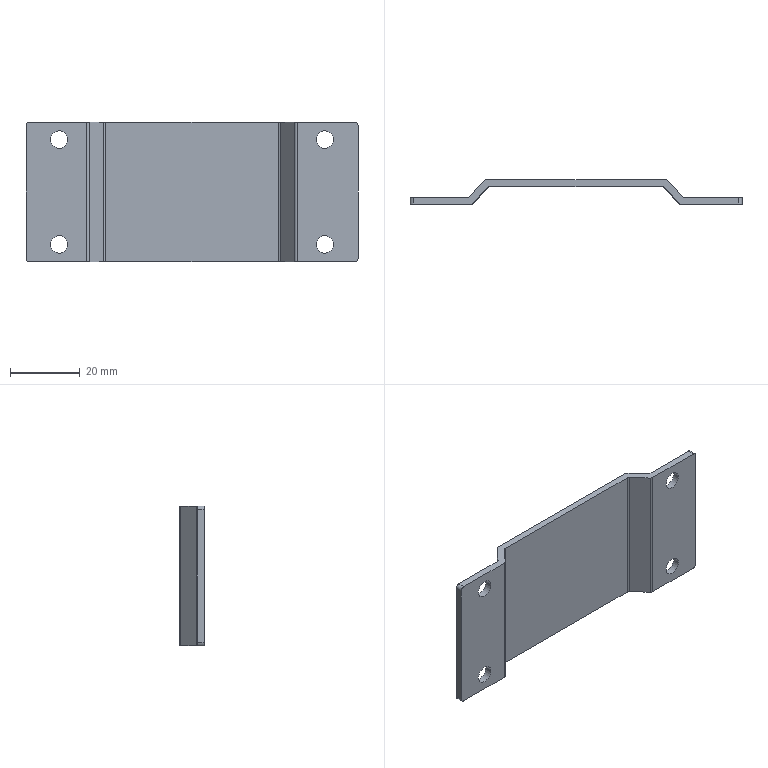Part | SolidWorks | features Extrusion 1, Fillet 1, ICE 1 | 1 solid | 34 faces | box 95 x 7 x 40 mm | volume 7797 mm3 | cylinder 20 | plane 14 | commonest cylinder face diameters 2 x12 5 x8
STEP:
#1=CARTESIAN_POINT('',(-40.5,-2.,15.));
#2=VERTEX_POINT('',#1);
#3=CARTESIAN_POINT('',(-35.5,-2.,15.));
#4=VERTEX_POINT('',#3);
#5=CARTESIAN_POINT('',(-38.,-2.,15.));
#6=DIRECTION('',(0.,-1.,0.));
#7=DIRECTION('',(0.,0.,-1.));
#8=AXIS2_PLACEMENT_3D('',#5,#6,#7);
#9=CIRCLE('',#8,2.5);
#10=EDGE_CURVE('',#2,#4,#9,.T.);
#11=ORIENTED_EDGE('',*,*,#10,.T.);
#12=CARTESIAN_POINT('',(-35.5,0.,15.));
#13=VERTEX_POINT('',#12);
#14=CARTESIAN_POINT('',(-35.5,-20.,15.));
#15=DIRECTION('',(0.,1.,0.));
#16=VECTOR('',#15,1000.);
#17=LINE('',#14,#16);
#18=EDGE_CURVE('',#4,#13,#17,.T.);
#19=ORIENTED_EDGE('',*,*,#18,.T.);
#20=CARTESIAN_POINT('',(-40.5,0.,15.));
#21=VERTEX_POINT('',#20);
#22=CARTESIAN_POINT('',(-38.,0.,15.));
#23=DIRECTION('',(0.,1.,0.));
#24=DIRECTION('',(1.,0.,0.));
#25=AXIS2_PLACEMENT_3D('',#22,#23,#24);
#26=CIRCLE('',#25,2.5);
#27=EDGE_CURVE('',#13,#21,#26,.T.);
#28=ORIENTED_EDGE('',*,*,#27,.T.);
#29=CARTESIAN_POINT('',(-40.5,-20.,15.));
#30=DIRECTION('',(0.,1.,0.));
#31=VECTOR('',#30,1000.);
#32=LINE('',#29,#31);
#33=EDGE_CURVE('',#2,#21,#32,.T.);
#34=ORIENTED_EDGE('',*,*,#33,.F.);
#35=EDGE_LOOP('',(#11,#19,#28,#34));
#36=FACE_OUTER_BOUND('',#35,.T.);
#37=CARTESIAN_POINT('',(-38.,-20.,15.));
#38=DIRECTION('',(0.,1.,0.));
#39=DIRECTION('',(-1.,0.,0.));
#40=AXIS2_PLACEMENT_3D('',#37,#38,#39);
#41=CYLINDRICAL_SURFACE('',#40,2.5);
#42=ADVANCED_FACE('',(#36),#41,.F.);
#43=CARTESIAN_POINT('',(35.5,-2.,15.));
#44=VERTEX_POINT('',#43);
#45=CARTESIAN_POINT('',(40.5,-2.,15.));
#46=VERTEX_POINT('',#45);
#47=CARTESIAN_POINT('',(38.,-2.,15.));
#48=DIRECTION('',(0.,-1.,0.));
#49=DIRECTION('',(0.,0.,-1.));
#50=AXIS2_PLACEMENT_3D('',#47,#48,#49);
#51=CIRCLE('',#50,2.5);
#52=EDGE_CURVE('',#44,#46,#51,.T.);
#53=ORIENTED_EDGE('',*,*,#52,.T.);
#54=CARTESIAN_POINT('',(40.5,0.,15.));
#55=VERTEX_POINT('',#54);
#56=CARTESIAN_POINT('',(40.5,-20.,15.));
#57=DIRECTION('',(0.,1.,0.));
#58=VECTOR('',#57,1000.);
#59=LINE('',#56,#58);
#60=EDGE_CURVE('',#46,#55,#59,.T.);
#61=ORIENTED_EDGE('',*,*,#60,.T.);
#62=CARTESIAN_POINT('',(35.5,0.,15.));
#63=VERTEX_POINT('',#62);
#64=CARTESIAN_POINT('',(38.,0.,15.));
#65=DIRECTION('',(0.,1.,0.));
#66=DIRECTION('',(-1.,0.,0.));
#67=AXIS2_PLACEMENT_3D('',#64,#65,#66);
#68=CIRCLE('',#67,2.5);
#69=EDGE_CURVE('',#55,#63,#68,.T.);
#70=ORIENTED_EDGE('',*,*,#69,.T.);
#71=CARTESIAN_POINT('',(35.5,-20.,15.));
#72=DIRECTION('',(0.,1.,0.));
#73=VECTOR('',#72,1000.);
#74=LINE('',#71,#73);
#75=EDGE_CURVE('',#44,#63,#74,.T.);
#76=ORIENTED_EDGE('',*,*,#75,.F.);
#77=EDGE_LOOP('',(#53,#61,#70,#76));
#78=FACE_OUTER_BOUND('',#77,.T.);
#79=CARTESIAN_POINT('',(38.,-20.,15.));
#80=DIRECTION('',(0.,1.,0.));
#81=DIRECTION('',(-1.,0.,0.));
#82=AXIS2_PLACEMENT_3D('',#79,#80,#81);
#83=CYLINDRICAL_SURFACE('',#82,2.5);
#84=ADVANCED_FACE('',(#78),#83,.F.);
#85=CARTESIAN_POINT('',(35.5,-2.,-15.));
#86=VERTEX_POINT('',#85);
#87=CARTESIAN_POINT('',(40.5,-2.,-15.));
#88=VERTEX_POINT('',#87);
#89=CARTESIAN_POINT('',(38.,-2.,-15.));
#90=DIRECTION('',(0.,-1.,0.));
#91=DIRECTION('',(0.,0.,-1.));
#92=AXIS2_PLACEMENT_3D('',#89,#90,#91);
#93=CIRCLE('',#92,2.5);
#94=EDGE_CURVE('',#86,#88,#93,.T.);
#95=ORIENTED_EDGE('',*,*,#94,.T.);
#96=CARTESIAN_POINT('',(40.5,0.,-15.));
#97=VERTEX_POINT('',#96);
#98=CARTESIAN_POINT('',(40.5,-20.,-15.));
#99=DIRECTION('',(0.,1.,0.));
#100=VECTOR('',#99,1000.);
#101=LINE('',#98,#100);
#102=EDGE_CURVE('',#88,#97,#101,.T.);
#103=ORIENTED_EDGE('',*,*,#102,.T.);
#104=CARTESIAN_POINT('',(35.5,0.,-15.));
#105=VERTEX_POINT('',#104);
#106=CARTESIAN_POINT('',(38.,0.,-15.));
#107=DIRECTION('',(0.,1.,0.));
#108=DIRECTION('',(1.,0.,0.));
#109=AXIS2_PLACEMENT_3D('',#106,#107,#108);
#110=CIRCLE('',#109,2.5);
#111=EDGE_CURVE('',#97,#105,#110,.T.);
#112=ORIENTED_EDGE('',*,*,#111,.T.);
#113=CARTESIAN_POINT('',(35.5,-20.,-15.));
#114=DIRECTION('',(0.,1.,0.));
#115=VECTOR('',#114,1000.);
#116=LINE('',#113,#115);
#117=EDGE_CURVE('',#86,#105,#116,.T.);
#118=ORIENTED_EDGE('',*,*,#117,.F.);
#119=EDGE_LOOP('',(#95,#103,#112,#118));
#120=FACE_OUTER_BOUND('',#119,.T.);
#121=CARTESIAN_POINT('',(38.,-20.,-15.));
#122=DIRECTION('',(0.,1.,0.));
#123=DIRECTION('',(-1.,0.,0.));
#124=AXIS2_PLACEMENT_3D('',#121,#122,#123);
#125=CYLINDRICAL_SURFACE('',#124,2.5);
#126=ADVANCED_FACE('',(#120),#125,.F.);
#127=CARTESIAN_POINT('',(-40.5,-2.,-15.));
#128=VERTEX_POINT('',#127);
#129=CARTESIAN_POINT('',(-35.5,-2.,-15.));
#130=VERTEX_POINT('',#129);
#131=CARTESIAN_POINT('',(-38.,-2.,-15.));
#132=DIRECTION('',(0.,-1.,0.));
#133=DIRECTION('',(0.,0.,-1.));
#134=AXIS2_PLACEMENT_3D('',#131,#132,#133);
#135=CIRCLE('',#134,2.5);
#136=EDGE_CURVE('',#128,#130,#135,.T.);
#137=ORIENTED_EDGE('',*,*,#136,.T.);
#138=CARTESIAN_POINT('',(-35.5,0.,-15.));
#139=VERTEX_POINT('',#138);
#140=CARTESIAN_POINT('',(-35.5,-20.,-15.));
#141=DIRECTION('',(0.,1.,0.));
#142=VECTOR('',#141,1000.);
#143=LINE('',#140,#142);
#144=EDGE_CURVE('',#130,#139,#143,.T.);
#145=ORIENTED_EDGE('',*,*,#144,.T.);
#146=CARTESIAN_POINT('',(-40.5,0.,-15.));
#147=VERTEX_POINT('',#146);
#148=CARTESIAN_POINT('',(-38.,0.,-15.));
#149=DIRECTION('',(0.,1.,0.));
#150=DIRECTION('',(-1.,0.,0.));
#151=AXIS2_PLACEMENT_3D('',#148,#149,#150);
#152=CIRCLE('',#151,2.5);
#153=EDGE_CURVE('',#139,#147,#152,.T.);
#154=ORIENTED_EDGE('',*,*,#153,.T.);
#155=CARTESIAN_POINT('',(-40.5,-20.,-15.));
#156=DIRECTION('',(0.,1.,0.));
#157=VECTOR('',#156,1000.);
#158=LINE('',#155,#157);
#159=EDGE_CURVE('',#128,#147,#158,.T.);
#160=ORIENTED_EDGE('',*,*,#159,.F.);
#161=EDGE_LOOP('',(#137,#145,#154,#160));
#162=FACE_OUTER_BOUND('',#161,.T.);
#163=CARTESIAN_POINT('',(-38.,-20.,-15.));
#164=DIRECTION('',(0.,1.,0.));
#165=DIRECTION('',(-1.,0.,0.));
#166=AXIS2_PLACEMENT_3D('',#163,#164,#165);
#167=CYLINDRICAL_SURFACE('',#166,2.5);
#168=ADVANCED_FACE('',(#162),#167,.F.);
#169=CARTESIAN_POINT('',(-47.5,0.,-19.));
#170=VERTEX_POINT('',#169);
#171=CARTESIAN_POINT('',(-47.5,0.,19.));
#172=VERTEX_POINT('',#171);
#173=CARTESIAN_POINT('',(-47.5,0.,-20.));
#174=DIRECTION('',(0.,0.,1.));
#175=VECTOR('',#174,1000.);
#176=LINE('',#173,#175);
#177=EDGE_CURVE('',#170,#172,#176,.T.);
#178=ORIENTED_EDGE('',*,*,#177,.F.);
#179=CARTESIAN_POINT('',(-47.5,-2.,-19.));
#180=VERTEX_POINT('',#179);
#181=CARTESIAN_POINT('',(-47.5,-2.,-19.));
#182=DIRECTION('',(0.,-1.,0.));
#183=VECTOR('',#182,1000.);
#184=LINE('',#181,#183);
#185=EDGE_CURVE('',#170,#180,#184,.T.);
#186=ORIENTED_EDGE('',*,*,#185,.T.);
#187=CARTESIAN_POINT('',(-47.5,-2.,19.));
#188=VERTEX_POINT('',#187);
#189=CARTESIAN_POINT('',(-47.5,-2.,-20.));
#190=DIRECTION('',(0.,0.,1.));
#191=VECTOR('',#190,1000.);
#192=LINE('',#189,#191);
#193=EDGE_CURVE('',#180,#188,#192,.T.);
#194=ORIENTED_EDGE('',*,*,#193,.T.);
#195=CARTESIAN_POINT('',(-47.5,-2.,19.));
#196=DIRECTION('',(0.,1.,0.));
#197=VECTOR('',#196,1000.);
#198=LINE('',#195,#197);
#199=EDGE_CURVE('',#188,#172,#198,.T.);
#200=ORIENTED_EDGE('',*,*,#199,.T.);
#201=EDGE_LOOP('',(#178,#186,#194,#200));
#202=FACE_OUTER_BOUND('',#201,.T.);
#203=CARTESIAN_POINT('',(-47.5,-2.,-20.));
#204=DIRECTION('',(-1.,0.,0.));
#205=DIRECTION('',(0.,0.,1.));
#206=AXIS2_PLACEMENT_3D('',#203,#204,#205);
#207=PLANE('',#206);
#208=ADVANCED_FACE('',(#202),#207,.T.);
#209=CARTESIAN_POINT('',(-38.,0.,15.));
#210=DIRECTION('',(0.,1.,0.));
#211=DIRECTION('',(1.,0.,0.));
#212=AXIS2_PLACEMENT_3D('',#209,#210,#211);
#213=CIRCLE('',#212,2.5);
#214=EDGE_CURVE('',#21,#13,#213,.T.);
#215=ORIENTED_EDGE('',*,*,#214,.F.);
#216=ORIENTED_EDGE('',*,*,#27,.F.);
#217=EDGE_LOOP('',(#215,#216));
#218=FACE_BOUND('',#217,.T.);
#219=CARTESIAN_POINT('',(-38.,0.,-15.));
#220=DIRECTION('',(0.,1.,0.));
#221=DIRECTION('',(-1.,0.,0.));
#222=AXIS2_PLACEMENT_3D('',#219,#220,#221);
#223=CIRCLE('',#222,2.5);
#224=EDGE_CURVE('',#147,#139,#223,.T.);
#225=ORIENTED_EDGE('',*,*,#224,.F.);
#226=ORIENTED_EDGE('',*,*,#153,.F.);
#227=EDGE_LOOP('',(#225,#226));
#228=FACE_BOUND('',#227,.T.);
#229=CARTESIAN_POINT('',(-30.945,0.,-20.));
#230=VERTEX_POINT('',#229);
#231=CARTESIAN_POINT('',(-46.5,0.,-20.));
#232=VERTEX_POINT('',#231);
#233=CARTESIAN_POINT('',(-47.5,0.,-20.));
#234=DIRECTION('',(-1.,0.,0.));
#235=VECTOR('',#234,1000.);
#236=LINE('',#233,#235);
#237=EDGE_CURVE('',#230,#232,#236,.T.);
#238=ORIENTED_EDGE('',*,*,#237,.T.);
#239=CARTESIAN_POINT('',(-46.5,0.,-19.));
#240=DIRECTION('',(0.,1.,0.));
#241=DIRECTION('',(0.,0.,1.));
#242=AXIS2_PLACEMENT_3D('',#239,#240,#241);
#243=CIRCLE('',#242,1.);
#244=EDGE_CURVE('',#232,#170,#243,.T.);
#245=ORIENTED_EDGE('',*,*,#244,.T.);
#246=ORIENTED_EDGE('',*,*,#177,.T.);
#247=CARTESIAN_POINT('',(-46.5,0.,20.));
#248=VERTEX_POINT('',#247);
#249=CARTESIAN_POINT('',(-46.5,0.,19.));
#250=DIRECTION('',(0.,1.,0.));
#251=DIRECTION('',(0.,0.,1.));
#252=AXIS2_PLACEMENT_3D('',#249,#250,#251);
#253=CIRCLE('',#252,1.);
#254=EDGE_CURVE('',#172,#248,#253,.T.);
#255=ORIENTED_EDGE('',*,*,#254,.T.);
#256=CARTESIAN_POINT('',(-30.945,0.,20.));
#257=VERTEX_POINT('',#256);
#258=CARTESIAN_POINT('',(-47.5,0.,20.));
#259=DIRECTION('',(-1.,0.,0.));
#260=VECTOR('',#259,1000.);
#261=LINE('',#258,#260);
#262=EDGE_CURVE('',#257,#248,#261,.T.);
#263=ORIENTED_EDGE('',*,*,#262,.F.);
#264=CARTESIAN_POINT('',(-30.945,0.,-20.));
#265=DIRECTION('',(0.,0.,1.));
#266=VECTOR('',#265,1000.);
#267=LINE('',#264,#266);
#268=EDGE_CURVE('',#230,#257,#267,.T.);
#269=ORIENTED_EDGE('',*,*,#268,.F.);
#270=EDGE_LOOP('',(#238,#245,#246,#255,#263,#269));
#271=FACE_OUTER_BOUND('',#270,.T.);
#272=CARTESIAN_POINT('',(-47.5,0.,-20.));
#273=DIRECTION('',(0.,1.,0.));
#274=DIRECTION('',(0.,0.,1.));
#275=AXIS2_PLACEMENT_3D('',#272,#273,#274);
#276=PLANE('',#275);
#277=ADVANCED_FACE('',(#218,#228,#271),#276,.T.);
#278=ORIENTED_EDGE('',*,*,#268,.T.);
#279=CARTESIAN_POINT('',(-30.202,0.331,20.));
#280=VERTEX_POINT('',#279);
#281=CARTESIAN_POINT('',(-30.945,1.,20.));
#282=DIRECTION('',(0.,0.,-1.));
#283=DIRECTION('',(1.,0.,0.));
#284=AXIS2_PLACEMENT_3D('',#281,#282,#283);
#285=CIRCLE('',#284,1.);
#286=EDGE_CURVE('',#280,#257,#285,.T.);
#287=ORIENTED_EDGE('',*,*,#286,.F.);
#288=CARTESIAN_POINT('',(-30.202,0.331,-20.));
#289=VERTEX_POINT('',#288);
#290=CARTESIAN_POINT('',(-30.202,0.331,-20.));
#291=DIRECTION('',(0.,0.,1.));
#292=VECTOR('',#291,1000.);
#293=LINE('',#290,#292);
#294=EDGE_CURVE('',#289,#280,#293,.T.);
#295=ORIENTED_EDGE('',*,*,#294,.F.);
#296=CARTESIAN_POINT('',(-30.945,1.,-20.));
#297=DIRECTION('',(0.,0.,-1.));
#298=DIRECTION('',(1.,0.,0.));
#299=AXIS2_PLACEMENT_3D('',#296,#297,#298);
#300=CIRCLE('',#299,1.);
#301=EDGE_CURVE('',#289,#230,#300,.T.);
#302=ORIENTED_EDGE('',*,*,#301,.T.);
#303=EDGE_LOOP('',(#278,#287,#295,#302));
#304=FACE_OUTER_BOUND('',#303,.T.);
#305=CARTESIAN_POINT('',(-30.945,1.,-20.));
#306=DIRECTION('',(0.,0.,1.));
#307=DIRECTION('',(1.,0.,0.));
#308=AXIS2_PLACEMENT_3D('',#305,#306,#307);
#309=CYLINDRICAL_SURFACE('',#308,1.);
#310=ADVANCED_FACE('',(#304),#309,.F.);
#311=ORIENTED_EDGE('',*,*,#294,.T.);
#312=CARTESIAN_POINT('',(-26.298,4.669,20.));
#313=VERTEX_POINT('',#312);
#314=CARTESIAN_POINT('',(-30.202,0.331,20.));
#315=DIRECTION('',(-0.669,-0.7433,0.));
#316=VECTOR('',#315,1000.);
#317=LINE('',#314,#316);
#318=EDGE_CURVE('',#313,#280,#317,.T.);
#319=ORIENTED_EDGE('',*,*,#318,.F.);
#320=CARTESIAN_POINT('',(-26.298,4.669,-20.));
#321=VERTEX_POINT('',#320);
#322=CARTESIAN_POINT('',(-26.298,4.669,-20.));
#323=DIRECTION('',(0.,0.,1.));
#324=VECTOR('',#323,1000.);
#325=LINE('',#322,#324);
#326=EDGE_CURVE('',#321,#313,#325,.T.);
#327=ORIENTED_EDGE('',*,*,#326,.F.);
#328=CARTESIAN_POINT('',(-30.202,0.331,-20.));
#329=DIRECTION('',(-0.669,-0.7433,0.));
#330=VECTOR('',#329,1000.);
#331=LINE('',#328,#330);
#332=EDGE_CURVE('',#321,#289,#331,.T.);
#333=ORIENTED_EDGE('',*,*,#332,.T.);
#334=EDGE_LOOP('',(#311,#319,#327,#333));
#335=FACE_OUTER_BOUND('',#334,.T.);
#336=CARTESIAN_POINT('',(-30.202,0.331,-20.));
#337=DIRECTION('',(-0.7433,0.669,0.));
#338=DIRECTION('',(-0.669,-0.7433,0.));
#339=AXIS2_PLACEMENT_3D('',#336,#337,#338);
#340=PLANE('',#339);
#341=ADVANCED_FACE('',(#335),#340,.T.);
#342=ORIENTED_EDGE('',*,*,#326,.T.);
#343=CARTESIAN_POINT('',(-25.555,5.,20.));
#344=VERTEX_POINT('',#343);
#345=CARTESIAN_POINT('',(-25.555,4.,20.));
#346=DIRECTION('',(0.,0.,1.));
#347=DIRECTION('',(-1.,0.,0.));
#348=AXIS2_PLACEMENT_3D('',#345,#346,#347);
#349=CIRCLE('',#348,1.);
#350=EDGE_CURVE('',#344,#313,#349,.T.);
#351=ORIENTED_EDGE('',*,*,#350,.F.);
#352=CARTESIAN_POINT('',(-25.555,5.,-20.));
#353=VERTEX_POINT('',#352);
#354=CARTESIAN_POINT('',(-25.555,5.,-20.));
#355=DIRECTION('',(0.,0.,1.));
#356=VECTOR('',#355,1000.);
#357=LINE('',#354,#356);
#358=EDGE_CURVE('',#353,#344,#357,.T.);
#359=ORIENTED_EDGE('',*,*,#358,.F.);
#360=CARTESIAN_POINT('',(-25.555,4.,-20.));
#361=DIRECTION('',(0.,0.,1.));
#362=DIRECTION('',(-1.,0.,0.));
#363=AXIS2_PLACEMENT_3D('',#360,#361,#362);
#364=CIRCLE('',#363,1.);
#365=EDGE_CURVE('',#353,#321,#364,.T.);
#366=ORIENTED_EDGE('',*,*,#365,.T.);
#367=EDGE_LOOP('',(#342,#351,#359,#366));
#368=FACE_OUTER_BOUND('',#367,.T.);
#369=CARTESIAN_POINT('',(-25.555,4.,-20.));
#370=DIRECTION('',(0.,0.,1.));
#371=DIRECTION('',(1.,0.,0.));
#372=AXIS2_PLACEMENT_3D('',#369,#370,#371);
#373=CYLINDRICAL_SURFACE('',#372,1.);
#374=ADVANCED_FACE('',(#368),#373,.T.);
#375=ORIENTED_EDGE('',*,*,#358,.T.);
#376=CARTESIAN_POINT('',(25.555,5.,20.));
#377=VERTEX_POINT('',#376);
#378=CARTESIAN_POINT('',(-25.555,5.,20.));
#379=DIRECTION('',(-1.,0.,0.));
#380=VECTOR('',#379,1000.);
#381=LINE('',#378,#380);
#382=EDGE_CURVE('',#377,#344,#381,.T.);
#383=ORIENTED_EDGE('',*,*,#382,.F.);
#384=CARTESIAN_POINT('',(25.555,5.,-20.));
#385=VERTEX_POINT('',#384);
#386=CARTESIAN_POINT('',(25.555,5.,-20.));
#387=DIRECTION('',(0.,0.,1.));
#388=VECTOR('',#387,1000.);
#389=LINE('',#386,#388);
#390=EDGE_CURVE('',#385,#377,#389,.T.);
#391=ORIENTED_EDGE('',*,*,#390,.F.);
#392=CARTESIAN_POINT('',(-25.555,5.,-20.));
#393=DIRECTION('',(-1.,0.,0.));
#394=VECTOR('',#393,1000.);
#395=LINE('',#392,#394);
#396=EDGE_CURVE('',#385,#353,#395,.T.);
#397=ORIENTED_EDGE('',*,*,#396,.T.);
#398=EDGE_LOOP('',(#375,#383,#391,#397));
#399=FACE_OUTER_BOUND('',#398,.T.);
#400=CARTESIAN_POINT('',(-25.555,5.,-20.));
#401=DIRECTION('',(0.,1.,0.));
#402=DIRECTION('',(0.,0.,1.));
#403=AXIS2_PLACEMENT_3D('',#400,#401,#402);
#404=PLANE('',#403);
#405=ADVANCED_FACE('',(#399),#404,.T.);
#406=ORIENTED_EDGE('',*,*,#390,.T.);
#407=CARTESIAN_POINT('',(26.298,4.669,20.));
#408=VERTEX_POINT('',#407);
#409=CARTESIAN_POINT('',(25.555,4.,20.));
#410=DIRECTION('',(0.,0.,1.));
#411=DIRECTION('',(-1.,0.,0.));
#412=AXIS2_PLACEMENT_3D('',#409,#410,#411);
#413=CIRCLE('',#412,1.);
#414=EDGE_CURVE('',#408,#377,#413,.T.);
#415=ORIENTED_EDGE('',*,*,#414,.F.);
#416=CARTESIAN_POINT('',(26.298,4.669,-20.));
#417=VERTEX_POINT('',#416);
#418=CARTESIAN_POINT('',(26.298,4.669,-20.));
#419=DIRECTION('',(0.,0.,1.));
#420=VECTOR('',#419,1000.);
#421=LINE('',#418,#420);
#422=EDGE_CURVE('',#417,#408,#421,.T.);
#423=ORIENTED_EDGE('',*,*,#422,.F.);
#424=CARTESIAN_POINT('',(25.555,4.,-20.));
#425=DIRECTION('',(0.,0.,1.));
#426=DIRECTION('',(-1.,0.,0.));
#427=AXIS2_PLACEMENT_3D('',#424,#425,#426);
#428=CIRCLE('',#427,1.);
#429=EDGE_CURVE('',#417,#385,#428,.T.);
#430=ORIENTED_EDGE('',*,*,#429,.T.);
#431=EDGE_LOOP('',(#406,#415,#423,#430));
#432=FACE_OUTER_BOUND('',#431,.T.);
#433=CARTESIAN_POINT('',(25.555,4.,-20.));
#434=DIRECTION('',(0.,0.,1.));
#435=DIRECTION('',(1.,0.,0.));
#436=AXIS2_PLACEMENT_3D('',#433,#434,#435);
#437=CYLINDRICAL_SURFACE('',#436,1.);
#438=ADVANCED_FACE('',(#432),#437,.T.);
#439=ORIENTED_EDGE('',*,*,#422,.T.);
#440=CARTESIAN_POINT('',(30.202,0.331,20.));
#441=VERTEX_POINT('',#440);
#442=CARTESIAN_POINT('',(26.298,4.669,20.));
#443=DIRECTION('',(-0.669,0.7433,0.));
#444=VECTOR('',#443,1000.);
#445=LINE('',#442,#444);
#446=EDGE_CURVE('',#441,#408,#445,.T.);
#447=ORIENTED_EDGE('',*,*,#446,.F.);
#448=CARTESIAN_POINT('',(30.202,0.331,-20.));
#449=VERTEX_POINT('',#448);
#450=CARTESIAN_POINT('',(30.202,0.331,-20.));
#451=DIRECTION('',(0.,0.,1.));
#452=VECTOR('',#451,1000.);
#453=LINE('',#450,#452);
#454=EDGE_CURVE('',#449,#441,#453,.T.);
#455=ORIENTED_EDGE('',*,*,#454,.F.);
#456=CARTESIAN_POINT('',(26.298,4.669,-20.));
#457=DIRECTION('',(-0.669,0.7433,0.));
#458=VECTOR('',#457,1000.);
#459=LINE('',#456,#458);
#460=EDGE_CURVE('',#449,#417,#459,.T.);
#461=ORIENTED_EDGE('',*,*,#460,.T.);
#462=EDGE_LOOP('',(#439,#447,#455,#461));
#463=FACE_OUTER_BOUND('',#462,.T.);
#464=CARTESIAN_POINT('',(26.298,4.669,-20.));
#465=DIRECTION('',(0.7433,0.669,0.));
#466=DIRECTION('',(-0.669,0.7433,0.));
#467=AXIS2_PLACEMENT_3D('',#464,#465,#466);
#468=PLANE('',#467);
#469=ADVANCED_FACE('',(#463),#468,.T.);
#470=ORIENTED_EDGE('',*,*,#454,.T.);
#471=CARTESIAN_POINT('',(30.945,0.,20.));
#472=VERTEX_POINT('',#471);
#473=CARTESIAN_POINT('',(30.945,1.,20.));
#474=DIRECTION('',(0.,0.,-1.));
#475=DIRECTION('',(1.,0.,0.));
#476=AXIS2_PLACEMENT_3D('',#473,#474,#475);
#477=CIRCLE('',#476,1.);
#478=EDGE_CURVE('',#472,#441,#477,.T.);
#479=ORIENTED_EDGE('',*,*,#478,.F.);
#480=CARTESIAN_POINT('',(30.945,0.,-20.));
#481=VERTEX_POINT('',#480);
#482=CARTESIAN_POINT('',(30.945,0.,-20.));
#483=DIRECTION('',(0.,0.,1.));
#484=VECTOR('',#483,1000.);
#485=LINE('',#482,#484);
#486=EDGE_CURVE('',#481,#472,#485,.T.);
#487=ORIENTED_EDGE('',*,*,#486,.F.);
#488=CARTESIAN_POINT('',(30.945,1.,-20.));
#489=DIRECTION('',(0.,0.,-1.));
#490=DIRECTION('',(1.,0.,0.));
#491=AXIS2_PLACEMENT_3D('',#488,#489,#490);
#492=CIRCLE('',#491,1.);
#493=EDGE_CURVE('',#481,#449,#492,.T.);
#494=ORIENTED_EDGE('',*,*,#493,.T.);
#495=EDGE_LOOP('',(#470,#479,#487,#494));
#496=FACE_OUTER_BOUND('',#495,.T.);
#497=CARTESIAN_POINT('',(30.945,1.,-20.));
#498=DIRECTION('',(0.,0.,1.));
#499=DIRECTION('',(1.,0.,0.));
#500=AXIS2_PLACEMENT_3D('',#497,#498,#499);
#501=CYLINDRICAL_SURFACE('',#500,1.);
#502=ADVANCED_FACE('',(#496),#501,.F.);
#503=CARTESIAN_POINT('',(38.,0.,15.));
#504=DIRECTION('',(0.,1.,0.));
#505=DIRECTION('',(-1.,0.,0.));
#506=AXIS2_PLACEMENT_3D('',#503,#504,#505);
#507=CIRCLE('',#506,2.5);
#508=EDGE_CURVE('',#63,#55,#507,.T.);
#509=ORIENTED_EDGE('',*,*,#508,.F.);
#510=ORIENTED_EDGE('',*,*,#69,.F.);
#511=EDGE_LOOP('',(#509,#510));
#512=FACE_BOUND('',#511,.T.);
#513=CARTESIAN_POINT('',(38.,0.,-15.));
#514=DIRECTION('',(0.,1.,0.));
#515=DIRECTION('',(1.,0.,0.));
#516=AXIS2_PLACEMENT_3D('',#513,#514,#515);
#517=CIRCLE('',#516,2.5);
#518=EDGE_CURVE('',#105,#97,#517,.T.);
#519=ORIENTED_EDGE('',*,*,#518,.F.);
#520=ORIENTED_EDGE('',*,*,#111,.F.);
#521=EDGE_LOOP('',(#519,#520));
#522=FACE_BOUND('',#521,.T.);
#523=CARTESIAN_POINT('',(47.5,0.,-19.));
#524=VERTEX_POINT('',#523);
#525=CARTESIAN_POINT('',(47.5,0.,19.));
#526=VERTEX_POINT('',#525);
#527=CARTESIAN_POINT('',(47.5,0.,-20.));
#528=DIRECTION('',(0.,0.,1.));
#529=VECTOR('',#528,1000.);
#530=LINE('',#527,#529);
#531=EDGE_CURVE('',#524,#526,#530,.T.);
#532=ORIENTED_EDGE('',*,*,#531,.F.);
#533=CARTESIAN_POINT('',(46.5,0.,-20.));
#534=VERTEX_POINT('',#533);
#535=CARTESIAN_POINT('',(46.5,0.,-19.));
#536=DIRECTION('',(0.,1.,0.));
#537=DIRECTION('',(-1.,0.,0.));
#538=AXIS2_PLACEMENT_3D('',#535,#536,#537);
#539=CIRCLE('',#538,1.);
#540=EDGE_CURVE('',#524,#534,#539,.T.);
#541=ORIENTED_EDGE('',*,*,#540,.T.);
#542=CARTESIAN_POINT('',(30.945,0.,-20.));
#543=DIRECTION('',(-1.,0.,0.));
#544=VECTOR('',#543,1000.);
#545=LINE('',#542,#544);
#546=EDGE_CURVE('',#534,#481,#545,.T.);
#547=ORIENTED_EDGE('',*,*,#546,.T.);
#548=ORIENTED_EDGE('',*,*,#486,.T.);
#549=CARTESIAN_POINT('',(46.5,0.,20.));
#550=VERTEX_POINT('',#549);
#551=CARTESIAN_POINT('',(30.945,0.,20.));
#552=DIRECTION('',(-1.,0.,0.));
#553=VECTOR('',#552,1000.);
#554=LINE('',#551,#553);
#555=EDGE_CURVE('',#550,#472,#554,.T.);
#556=ORIENTED_EDGE('',*,*,#555,.F.);
#557=CARTESIAN_POINT('',(46.5,0.,19.));
#558=DIRECTION('',(0.,1.,0.));
#559=DIRECTION('',(-1.,0.,0.));
#560=AXIS2_PLACEMENT_3D('',#557,#558,#559);
#561=CIRCLE('',#560,1.);
#562=EDGE_CURVE('',#550,#526,#561,.T.);
#563=ORIENTED_EDGE('',*,*,#562,.T.);
#564=EDGE_LOOP('',(#532,#541,#547,#548,#556,#563));
#565=FACE_OUTER_BOUND('',#564,.T.);
#566=CARTESIAN_POINT('',(30.945,0.,-20.));
#567=DIRECTION('',(0.,1.,0.));
#568=DIRECTION('',(-1.,0.,0.));
#569=AXIS2_PLACEMENT_3D('',#566,#567,#568);
#570=PLANE('',#569);
#571=ADVANCED_FACE('',(#512,#522,#565),#570,.T.);
#572=CARTESIAN_POINT('',(47.5,-2.,-19.));
#573=VERTEX_POINT('',#572);
#574=CARTESIAN_POINT('',(47.5,-2.,19.));
#575=VERTEX_POINT('',#574);
#576=CARTESIAN_POINT('',(47.5,-2.,-20.));
#577=DIRECTION('',(0.,0.,1.));
#578=VECTOR('',#577,1000.);
#579=LINE('',#576,#578);
#580=EDGE_CURVE('',#573,#575,#579,.T.);
#581=ORIENTED_EDGE('',*,*,#580,.F.);
#582=CARTESIAN_POINT('',(47.5,0.,-19.));
#583=DIRECTION('',(0.,1.,0.));
#584=VECTOR('',#583,1000.);
#585=LINE('',#582,#584);
#586=EDGE_CURVE('',#573,#524,#585,.T.);
#587=ORIENTED_EDGE('',*,*,#586,.T.);
#588=ORIENTED_EDGE('',*,*,#531,.T.);
#589=CARTESIAN_POINT('',(47.5,-2.,19.));
#590=DIRECTION('',(0.,-1.,0.));
#591=VECTOR('',#590,1000.);
#592=LINE('',#589,#591);
#593=EDGE_CURVE('',#526,#575,#592,.T.);
#594=ORIENTED_EDGE('',*,*,#593,.T.);
#595=EDGE_LOOP('',(#581,#587,#588,#594));
#596=FACE_OUTER_BOUND('',#595,.T.);
#597=CARTESIAN_POINT('',(47.5,-2.,-20.));
#598=DIRECTION('',(1.,0.,0.));
#599=DIRECTION('',(0.,0.,-1.));
#600=AXIS2_PLACEMENT_3D('',#597,#598,#599);
#601=PLANE('',#600);
#602=ADVANCED_FACE('',(#596),#601,.T.);
#603=ORIENTED_EDGE('',*,*,#52,.F.);
#604=CARTESIAN_POINT('',(38.,-2.,15.));
#605=DIRECTION('',(0.,-1.,0.));
#606=DIRECTION('',(0.,0.,-1.));
#607=AXIS2_PLACEMENT_3D('',#604,#605,#606);
#608=CIRCLE('',#607,2.5);
#609=EDGE_CURVE('',#46,#44,#608,.T.);
#610=ORIENTED_EDGE('',*,*,#609,.F.);
#611=EDGE_LOOP('',(#603,#610));
#612=FACE_BOUND('',#611,.T.);
#613=ORIENTED_EDGE('',*,*,#94,.F.);
#614=CARTESIAN_POINT('',(38.,-2.,-15.));
#615=DIRECTION('',(0.,-1.,0.));
#616=DIRECTION('',(0.,0.,-1.));
#617=AXIS2_PLACEMENT_3D('',#614,#615,#616);
#618=CIRCLE('',#617,2.5);
#619=EDGE_CURVE('',#88,#86,#618,.T.);
#620=ORIENTED_EDGE('',*,*,#619,.F.);
#621=EDGE_LOOP('',(#613,#620));
#622=FACE_BOUND('',#621,.T.);
#623=CARTESIAN_POINT('',(30.055,-2.,-20.));
#624=VERTEX_POINT('',#623);
#625=CARTESIAN_POINT('',(46.5,-2.,-20.));
#626=VERTEX_POINT('',#625);
#627=CARTESIAN_POINT('',(30.055,-2.,-20.));
#628=DIRECTION('',(1.,0.,0.));
#629=VECTOR('',#628,1000.);
#630=LINE('',#627,#629);
#631=EDGE_CURVE('',#624,#626,#630,.T.);
#632=ORIENTED_EDGE('',*,*,#631,.T.);
#633=CARTESIAN_POINT('',(46.5,-2.,-19.));
#634=DIRECTION('',(0.,-1.,0.));
#635=DIRECTION('',(0.,0.,-1.));
#636=AXIS2_PLACEMENT_3D('',#633,#634,#635);
#637=CIRCLE('',#636,1.);
#638=EDGE_CURVE('',#626,#573,#637,.T.);
#639=ORIENTED_EDGE('',*,*,#638,.T.);
#640=ORIENTED_EDGE('',*,*,#580,.T.);
#641=CARTESIAN_POINT('',(46.5,-2.,20.));
#642=VERTEX_POINT('',#641);
#643=CARTESIAN_POINT('',(46.5,-2.,19.));
#644=DIRECTION('',(0.,-1.,0.));
#645=DIRECTION('',(0.,0.,-1.));
#646=AXIS2_PLACEMENT_3D('',#643,#644,#645);
#647=CIRCLE('',#646,1.);
#648=EDGE_CURVE('',#575,#642,#647,.T.);
#649=ORIENTED_EDGE('',*,*,#648,.T.);
#650=CARTESIAN_POINT('',(30.055,-2.,20.));
#651=VERTEX_POINT('',#650);
#652=CARTESIAN_POINT('',(30.055,-2.,20.));
#653=DIRECTION('',(1.,0.,0.));
#654=VECTOR('',#653,1000.);
#655=LINE('',#652,#654);
#656=EDGE_CURVE('',#651,#642,#655,.T.);
#657=ORIENTED_EDGE('',*,*,#656,.F.);
#658=CARTESIAN_POINT('',(30.055,-2.,-20.));
#659=DIRECTION('',(0.,0.,1.));
#660=VECTOR('',#659,1000.);
#661=LINE('',#658,#660);
#662=EDGE_CURVE('',#624,#651,#661,.T.);
#663=ORIENTED_EDGE('',*,*,#662,.F.);
#664=EDGE_LOOP('',(#632,#639,#640,#649,#657,#663));
#665=FACE_OUTER_BOUND('',#664,.T.);
#666=CARTESIAN_POINT('',(30.055,-2.,-20.));
#667=DIRECTION('',(0.,-1.,0.));
#668=DIRECTION('',(0.,0.,-1.));
#669=AXIS2_PLACEMENT_3D('',#666,#667,#668);
#670=PLANE('',#669);
#671=ADVANCED_FACE('',(#612,#622,#665),#670,.T.);
#672=ORIENTED_EDGE('',*,*,#662,.T.);
#673=CARTESIAN_POINT('',(29.311,-1.669,20.));
#674=VERTEX_POINT('',#673);
#675=CARTESIAN_POINT('',(30.055,-1.,20.));
#676=DIRECTION('',(0.,0.,1.));
#677=DIRECTION('',(1.,0.,0.));
#678=AXIS2_PLACEMENT_3D('',#675,#676,#677);
#679=CIRCLE('',#678,1.);
#680=EDGE_CURVE('',#674,#651,#679,.T.);
#681=ORIENTED_EDGE('',*,*,#680,.F.);
#682=CARTESIAN_POINT('',(29.311,-1.669,-20.));
#683=VERTEX_POINT('',#682);
#684=CARTESIAN_POINT('',(29.311,-1.669,-20.));
#685=DIRECTION('',(0.,0.,1.));
#686=VECTOR('',#685,1000.);
#687=LINE('',#684,#686);
#688=EDGE_CURVE('',#683,#674,#687,.T.);
#689=ORIENTED_EDGE('',*,*,#688,.F.);
#690=CARTESIAN_POINT('',(30.055,-1.,-20.));
#691=DIRECTION('',(0.,0.,1.));
#692=DIRECTION('',(1.,0.,0.));
#693=AXIS2_PLACEMENT_3D('',#690,#691,#692);
#694=CIRCLE('',#693,1.);
#695=EDGE_CURVE('',#683,#624,#694,.T.);
#696=ORIENTED_EDGE('',*,*,#695,.T.);
#697=EDGE_LOOP('',(#672,#681,#689,#696));
#698=FACE_OUTER_BOUND('',#697,.T.);
#699=CARTESIAN_POINT('',(30.055,-1.,-20.));
#700=DIRECTION('',(0.,0.,1.));
#701=DIRECTION('',(1.,0.,0.));
#702=AXIS2_PLACEMENT_3D('',#699,#700,#701);
#703=CYLINDRICAL_SURFACE('',#702,1.);
#704=ADVANCED_FACE('',(#698),#703,.T.);
#705=ORIENTED_EDGE('',*,*,#688,.T.);
#706=CARTESIAN_POINT('',(25.407,2.669,20.));
#707=VERTEX_POINT('',#706);
#708=CARTESIAN_POINT('',(25.407,2.669,20.));
#709=DIRECTION('',(0.669,-0.7433,0.));
#710=VECTOR('',#709,1000.);
#711=LINE('',#708,#710);
#712=EDGE_CURVE('',#707,#674,#711,.T.);
#713=ORIENTED_EDGE('',*,*,#712,.F.);
#714=CARTESIAN_POINT('',(25.407,2.669,-20.));
#715=VERTEX_POINT('',#714);
#716=CARTESIAN_POINT('',(25.407,2.669,-20.));
#717=DIRECTION('',(0.,0.,1.));
#718=VECTOR('',#717,1000.);
#719=LINE('',#716,#718);
#720=EDGE_CURVE('',#715,#707,#719,.T.);
#721=ORIENTED_EDGE('',*,*,#720,.F.);
#722=CARTESIAN_POINT('',(25.407,2.669,-20.));
#723=DIRECTION('',(0.669,-0.7433,0.));
#724=VECTOR('',#723,1000.);
#725=LINE('',#722,#724);
#726=EDGE_CURVE('',#715,#683,#725,.T.);
#727=ORIENTED_EDGE('',*,*,#726,.T.);
#728=EDGE_LOOP('',(#705,#713,#721,#727));
#729=FACE_OUTER_BOUND('',#728,.T.);
#730=CARTESIAN_POINT('',(25.407,2.669,-20.));
#731=DIRECTION('',(-0.7433,-0.669,0.));
#732=DIRECTION('',(0.669,-0.7433,0.));
#733=AXIS2_PLACEMENT_3D('',#730,#731,#732);
#734=PLANE('',#733);
#735=ADVANCED_FACE('',(#729),#734,.T.);
#736=ORIENTED_EDGE('',*,*,#720,.T.);
#737=CARTESIAN_POINT('',(24.664,3.,20.));
#738=VERTEX_POINT('',#737);
#739=CARTESIAN_POINT('',(24.664,2.,20.));
#740=DIRECTION('',(0.,0.,-1.));
#741=DIRECTION('',(-1.,0.,0.));
#742=AXIS2_PLACEMENT_3D('',#739,#740,#741);
#743=CIRCLE('',#742,1.);
#744=EDGE_CURVE('',#738,#707,#743,.T.);
#745=ORIENTED_EDGE('',*,*,#744,.F.);
#746=CARTESIAN_POINT('',(24.664,3.,-20.));
#747=VERTEX_POINT('',#746);
#748=CARTESIAN_POINT('',(24.664,3.,-20.));
#749=DIRECTION('',(0.,0.,1.));
#750=VECTOR('',#749,1000.);
#751=LINE('',#748,#750);
#752=EDGE_CURVE('',#747,#738,#751,.T.);
#753=ORIENTED_EDGE('',*,*,#752,.F.);
#754=CARTESIAN_POINT('',(24.664,2.,-20.));
#755=DIRECTION('',(0.,0.,-1.));
#756=DIRECTION('',(-1.,0.,0.));
#757=AXIS2_PLACEMENT_3D('',#754,#755,#756);
#758=CIRCLE('',#757,1.);
#759=EDGE_CURVE('',#747,#715,#758,.T.);
#760=ORIENTED_EDGE('',*,*,#759,.T.);
#761=EDGE_LOOP('',(#736,#745,#753,#760));
#762=FACE_OUTER_BOUND('',#761,.T.);
#763=CARTESIAN_POINT('',(24.664,2.,-20.));
#764=DIRECTION('',(0.,0.,1.));
#765=DIRECTION('',(1.,0.,0.));
#766=AXIS2_PLACEMENT_3D('',#763,#764,#765);
#767=CYLINDRICAL_SURFACE('',#766,1.);
#768=ADVANCED_FACE('',(#762),#767,.F.);
#769=ORIENTED_EDGE('',*,*,#752,.T.);
#770=CARTESIAN_POINT('',(-24.664,3.,20.));
#771=VERTEX_POINT('',#770);
#772=CARTESIAN_POINT('',(-24.664,3.,20.));
#773=DIRECTION('',(1.,0.,0.));
#774=VECTOR('',#773,1000.);
#775=LINE('',#772,#774);
#776=EDGE_CURVE('',#771,#738,#775,.T.);
#777=ORIENTED_EDGE('',*,*,#776,.F.);
#778=CARTESIAN_POINT('',(-24.664,3.,-20.));
#779=VERTEX_POINT('',#778);
#780=CARTESIAN_POINT('',(-24.664,3.,-20.));
#781=DIRECTION('',(0.,0.,1.));
#782=VECTOR('',#781,1000.);
#783=LINE('',#780,#782);
#784=EDGE_CURVE('',#779,#771,#783,.T.);
#785=ORIENTED_EDGE('',*,*,#784,.F.);
#786=CARTESIAN_POINT('',(-24.664,3.,-20.));
#787=DIRECTION('',(1.,0.,0.));
#788=VECTOR('',#787,1000.);
#789=LINE('',#786,#788);
#790=EDGE_CURVE('',#779,#747,#789,.T.);
#791=ORIENTED_EDGE('',*,*,#790,.T.);
#792=EDGE_LOOP('',(#769,#777,#785,#791));
#793=FACE_OUTER_BOUND('',#792,.T.);
#794=CARTESIAN_POINT('',(-24.664,3.,-20.));
#795=DIRECTION('',(0.,-1.,0.));
#796=DIRECTION('',(0.,0.,-1.));
#797=AXIS2_PLACEMENT_3D('',#794,#795,#796);
#798=PLANE('',#797);
#799=ADVANCED_FACE('',(#793),#798,.T.);
#800=ORIENTED_EDGE('',*,*,#784,.T.);
#801=CARTESIAN_POINT('',(-25.407,2.669,20.));
#802=VERTEX_POINT('',#801);
#803=CARTESIAN_POINT('',(-24.664,2.,20.));
#804=DIRECTION('',(0.,0.,-1.));
#805=DIRECTION('',(-1.,0.,0.));
#806=AXIS2_PLACEMENT_3D('',#803,#804,#805);
#807=CIRCLE('',#806,1.);
#808=EDGE_CURVE('',#802,#771,#807,.T.);
#809=ORIENTED_EDGE('',*,*,#808,.F.);
#810=CARTESIAN_POINT('',(-25.407,2.669,-20.));
#811=VERTEX_POINT('',#810);
#812=CARTESIAN_POINT('',(-25.407,2.669,-20.));
#813=DIRECTION('',(0.,0.,1.));
#814=VECTOR('',#813,1000.);
#815=LINE('',#812,#814);
#816=EDGE_CURVE('',#811,#802,#815,.T.);
#817=ORIENTED_EDGE('',*,*,#816,.F.);
#818=CARTESIAN_POINT('',(-24.664,2.,-20.));
#819=DIRECTION('',(0.,0.,-1.));
#820=DIRECTION('',(-1.,0.,0.));
#821=AXIS2_PLACEMENT_3D('',#818,#819,#820);
#822=CIRCLE('',#821,1.);
#823=EDGE_CURVE('',#811,#779,#822,.T.);
#824=ORIENTED_EDGE('',*,*,#823,.T.);
#825=EDGE_LOOP('',(#800,#809,#817,#824));
#826=FACE_OUTER_BOUND('',#825,.T.);
#827=CARTESIAN_POINT('',(-24.664,2.,-20.));
#828=DIRECTION('',(0.,0.,1.));
#829=DIRECTION('',(1.,0.,0.));
#830=AXIS2_PLACEMENT_3D('',#827,#828,#829);
#831=CYLINDRICAL_SURFACE('',#830,1.);
#832=ADVANCED_FACE('',(#826),#831,.F.);
#833=ORIENTED_EDGE('',*,*,#816,.T.);
#834=CARTESIAN_POINT('',(-29.311,-1.669,20.));
#835=VERTEX_POINT('',#834);
#836=CARTESIAN_POINT('',(-29.311,-1.669,20.));
#837=DIRECTION('',(0.669,0.7433,0.));
#838=VECTOR('',#837,1000.);
#839=LINE('',#836,#838);
#840=EDGE_CURVE('',#835,#802,#839,.T.);
#841=ORIENTED_EDGE('',*,*,#840,.F.);
#842=CARTESIAN_POINT('',(-29.311,-1.669,-20.));
#843=VERTEX_POINT('',#842);
#844=CARTESIAN_POINT('',(-29.311,-1.669,-20.));
#845=DIRECTION('',(0.,0.,1.));
#846=VECTOR('',#845,1000.);
#847=LINE('',#844,#846);
#848=EDGE_CURVE('',#843,#835,#847,.T.);
#849=ORIENTED_EDGE('',*,*,#848,.F.);
#850=CARTESIAN_POINT('',(-29.311,-1.669,-20.));
#851=DIRECTION('',(0.669,0.7433,0.));
#852=VECTOR('',#851,1000.);
#853=LINE('',#850,#852);
#854=EDGE_CURVE('',#843,#811,#853,.T.);
#855=ORIENTED_EDGE('',*,*,#854,.T.);
#856=EDGE_LOOP('',(#833,#841,#849,#855));
#857=FACE_OUTER_BOUND('',#856,.T.);
#858=CARTESIAN_POINT('',(-29.311,-1.669,-20.));
#859=DIRECTION('',(0.7433,-0.669,0.));
#860=DIRECTION('',(0.669,0.7433,0.));
#861=AXIS2_PLACEMENT_3D('',#858,#859,#860);
#862=PLANE('',#861);
#863=ADVANCED_FACE('',(#857),#862,.T.);
#864=ORIENTED_EDGE('',*,*,#848,.T.);
#865=CARTESIAN_POINT('',(-30.055,-2.,20.));
#866=VERTEX_POINT('',#865);
#867=CARTESIAN_POINT('',(-30.055,-1.,20.));
#868=DIRECTION('',(0.,0.,1.));
#869=DIRECTION('',(1.,0.,0.));
#870=AXIS2_PLACEMENT_3D('',#867,#868,#869);
#871=CIRCLE('',#870,1.);
#872=EDGE_CURVE('',#866,#835,#871,.T.);
#873=ORIENTED_EDGE('',*,*,#872,.F.);
#874=CARTESIAN_POINT('',(-30.055,-2.,-20.));
#875=VERTEX_POINT('',#874);
#876=CARTESIAN_POINT('',(-30.055,-2.,-20.));
#877=DIRECTION('',(0.,0.,1.));
#878=VECTOR('',#877,1000.);
#879=LINE('',#876,#878);
#880=EDGE_CURVE('',#875,#866,#879,.T.);
#881=ORIENTED_EDGE('',*,*,#880,.F.);
#882=CARTESIAN_POINT('',(-30.055,-1.,-20.));
#883=DIRECTION('',(0.,0.,1.));
#884=DIRECTION('',(1.,0.,0.));
#885=AXIS2_PLACEMENT_3D('',#882,#883,#884);
#886=CIRCLE('',#885,1.);
#887=EDGE_CURVE('',#875,#843,#886,.T.);
#888=ORIENTED_EDGE('',*,*,#887,.T.);
#889=EDGE_LOOP('',(#864,#873,#881,#888));
#890=FACE_OUTER_BOUND('',#889,.T.);
#891=CARTESIAN_POINT('',(-30.055,-1.,-20.));
#892=DIRECTION('',(0.,0.,1.));
#893=DIRECTION('',(1.,0.,0.));
#894=AXIS2_PLACEMENT_3D('',#891,#892,#893);
#895=CYLINDRICAL_SURFACE('',#894,1.);
#896=ADVANCED_FACE('',(#890),#895,.T.);
#897=ORIENTED_EDGE('',*,*,#10,.F.);
#898=CARTESIAN_POINT('',(-38.,-2.,15.));
#899=DIRECTION('',(0.,-1.,0.));
#900=DIRECTION('',(0.,0.,-1.));
#901=AXIS2_PLACEMENT_3D('',#898,#899,#900);
#902=CIRCLE('',#901,2.5);
#903=EDGE_CURVE('',#4,#2,#902,.T.);
#904=ORIENTED_EDGE('',*,*,#903,.F.);
#905=EDGE_LOOP('',(#897,#904));
#906=FACE_BOUND('',#905,.T.);
#907=ORIENTED_EDGE('',*,*,#136,.F.);
#908=CARTESIAN_POINT('',(-38.,-2.,-15.));
#909=DIRECTION('',(0.,-1.,0.));
#910=DIRECTION('',(0.,0.,-1.));
#911=AXIS2_PLACEMENT_3D('',#908,#909,#910);
#912=CIRCLE('',#911,2.5);
#913=EDGE_CURVE('',#130,#128,#912,.T.);
#914=ORIENTED_EDGE('',*,*,#913,.F.);
#915=EDGE_LOOP('',(#907,#914));
#916=FACE_BOUND('',#915,.T.);
#917=ORIENTED_EDGE('',*,*,#193,.F.);
#918=CARTESIAN_POINT('',(-46.5,-2.,-20.));
#919=VERTEX_POINT('',#918);
#920=CARTESIAN_POINT('',(-46.5,-2.,-19.));
#921=DIRECTION('',(0.,-1.,0.));
#922=DIRECTION('',(0.,0.,-1.));
#923=AXIS2_PLACEMENT_3D('',#920,#921,#922);
#924=CIRCLE('',#923,1.);
#925=EDGE_CURVE('',#180,#919,#924,.T.);
#926=ORIENTED_EDGE('',*,*,#925,.T.);
#927=CARTESIAN_POINT('',(-47.5,-2.,-20.));
#928=DIRECTION('',(1.,0.,0.));
#929=VECTOR('',#928,1000.);
#930=LINE('',#927,#929);
#931=EDGE_CURVE('',#919,#875,#930,.T.);
#932=ORIENTED_EDGE('',*,*,#931,.T.);
#933=ORIENTED_EDGE('',*,*,#880,.T.);
#934=CARTESIAN_POINT('',(-46.5,-2.,20.));
#935=VERTEX_POINT('',#934);
#936=CARTESIAN_POINT('',(-47.5,-2.,20.));
#937=DIRECTION('',(1.,0.,0.));
#938=VECTOR('',#937,1000.);
#939=LINE('',#936,#938);
#940=EDGE_CURVE('',#935,#866,#939,.T.);
#941=ORIENTED_EDGE('',*,*,#940,.F.);
#942=CARTESIAN_POINT('',(-46.5,-2.,19.));
#943=DIRECTION('',(0.,-1.,0.));
#944=DIRECTION('',(0.,0.,-1.));
#945=AXIS2_PLACEMENT_3D('',#942,#943,#944);
#946=CIRCLE('',#945,1.);
#947=EDGE_CURVE('',#935,#188,#946,.T.);
#948=ORIENTED_EDGE('',*,*,#947,.T.);
#949=EDGE_LOOP('',(#917,#926,#932,#933,#941,#948));
#950=FACE_OUTER_BOUND('',#949,.T.);
#951=CARTESIAN_POINT('',(-47.5,-2.,-20.));
#952=DIRECTION('',(0.,-1.,0.));
#953=DIRECTION('',(0.,0.,-1.));
#954=AXIS2_PLACEMENT_3D('',#951,#952,#953);
#955=PLANE('',#954);
#956=ADVANCED_FACE('',(#906,#916,#950),#955,.T.);
#957=ORIENTED_EDGE('',*,*,#931,.F.);
#958=CARTESIAN_POINT('',(-46.5,0.,-20.));
#959=DIRECTION('',(0.,1.,0.));
#960=VECTOR('',#959,1000.);
#961=LINE('',#958,#960);
#962=EDGE_CURVE('',#919,#232,#961,.T.);
#963=ORIENTED_EDGE('',*,*,#962,.T.);
#964=ORIENTED_EDGE('',*,*,#237,.F.);
#965=ORIENTED_EDGE('',*,*,#301,.F.);
#966=ORIENTED_EDGE('',*,*,#332,.F.);
#967=ORIENTED_EDGE('',*,*,#365,.F.);
#968=ORIENTED_EDGE('',*,*,#396,.F.);
#969=ORIENTED_EDGE('',*,*,#429,.F.);
#970=ORIENTED_EDGE('',*,*,#460,.F.);
#971=ORIENTED_EDGE('',*,*,#493,.F.);
#972=ORIENTED_EDGE('',*,*,#546,.F.);
#973=CARTESIAN_POINT('',(46.5,-2.,-20.));
#974=DIRECTION('',(0.,-1.,0.));
#975=VECTOR('',#974,1000.);
#976=LINE('',#973,#975);
#977=EDGE_CURVE('',#534,#626,#976,.T.);
#978=ORIENTED_EDGE('',*,*,#977,.T.);
#979=ORIENTED_EDGE('',*,*,#631,.F.);
#980=ORIENTED_EDGE('',*,*,#695,.F.);
#981=ORIENTED_EDGE('',*,*,#726,.F.);
#982=ORIENTED_EDGE('',*,*,#759,.F.);
#983=ORIENTED_EDGE('',*,*,#790,.F.);
#984=ORIENTED_EDGE('',*,*,#823,.F.);
#985=ORIENTED_EDGE('',*,*,#854,.F.);
#986=ORIENTED_EDGE('',*,*,#887,.F.);
#987=EDGE_LOOP('',(#957,#963,#964,#965,#966,#967,#968,#969,#970,#971,#972,#978,#979,#980,#981,#982,#983,#984,#985,#986));
#988=FACE_OUTER_BOUND('',#987,.T.);
#989=CARTESIAN_POINT('',(-30.945,1.,-20.));
#990=DIRECTION('',(0.,0.,1.));
#991=DIRECTION('',(1.,0.,0.));
#992=AXIS2_PLACEMENT_3D('',#989,#990,#991);
#993=PLANE('',#992);
#994=ADVANCED_FACE('',(#988),#993,.F.);
#995=ORIENTED_EDGE('',*,*,#262,.T.);
#996=CARTESIAN_POINT('',(-46.5,1.,20.));
#997=DIRECTION('',(0.,-1.,0.));
#998=VECTOR('',#997,1000.);
#999=LINE('',#996,#998);
#1000=EDGE_CURVE('',#248,#935,#999,.T.);
#1001=ORIENTED_EDGE('',*,*,#1000,.T.);
#1002=ORIENTED_EDGE('',*,*,#940,.T.);
#1003=ORIENTED_EDGE('',*,*,#872,.T.);
#1004=ORIENTED_EDGE('',*,*,#840,.T.);
#1005=ORIENTED_EDGE('',*,*,#808,.T.);
#1006=ORIENTED_EDGE('',*,*,#776,.T.);
#1007=ORIENTED_EDGE('',*,*,#744,.T.);
#1008=ORIENTED_EDGE('',*,*,#712,.T.);
#1009=ORIENTED_EDGE('',*,*,#680,.T.);
#1010=ORIENTED_EDGE('',*,*,#656,.T.);
#1011=CARTESIAN_POINT('',(46.5,1.,20.));
#1012=DIRECTION('',(0.,1.,0.));
#1013=VECTOR('',#1012,1000.);
#1014=LINE('',#1011,#1013);
#1015=EDGE_CURVE('',#642,#550,#1014,.T.);
#1016=ORIENTED_EDGE('',*,*,#1015,.T.);
#1017=ORIENTED_EDGE('',*,*,#555,.T.);
#1018=ORIENTED_EDGE('',*,*,#478,.T.);
#1019=ORIENTED_EDGE('',*,*,#446,.T.);
#1020=ORIENTED_EDGE('',*,*,#414,.T.);
#1021=ORIENTED_EDGE('',*,*,#382,.T.);
#1022=ORIENTED_EDGE('',*,*,#350,.T.);
#1023=ORIENTED_EDGE('',*,*,#318,.T.);
#1024=ORIENTED_EDGE('',*,*,#286,.T.);
#1025=EDGE_LOOP('',(#995,#1001,#1002,#1003,#1004,#1005,#1006,#1007,#1008,#1009,#1010,#1016,#1017,#1018,#1019,#1020,#1021,#1022,#1023,#1024));
#1026=FACE_OUTER_BOUND('',#1025,.T.);
#1027=CARTESIAN_POINT('',(-30.945,1.,20.));
#1028=DIRECTION('',(0.,0.,1.));
#1029=DIRECTION('',(1.,0.,0.));
#1030=AXIS2_PLACEMENT_3D('',#1027,#1028,#1029);
#1031=PLANE('',#1030);
#1032=ADVANCED_FACE('',(#1026),#1031,.T.);
#1033=ORIENTED_EDGE('',*,*,#144,.F.);
#1034=ORIENTED_EDGE('',*,*,#913,.T.);
#1035=ORIENTED_EDGE('',*,*,#159,.T.);
#1036=ORIENTED_EDGE('',*,*,#224,.T.);
#1037=EDGE_LOOP('',(#1033,#1034,#1035,#1036));
#1038=FACE_OUTER_BOUND('',#1037,.T.);
#1039=CARTESIAN_POINT('',(-38.,-20.,-15.));
#1040=DIRECTION('',(0.,1.,0.));
#1041=DIRECTION('',(-1.,0.,0.));
#1042=AXIS2_PLACEMENT_3D('',#1039,#1040,#1041);
#1043=CYLINDRICAL_SURFACE('',#1042,2.5);
#1044=ADVANCED_FACE('',(#1038),#1043,.F.);
#1045=ORIENTED_EDGE('',*,*,#102,.F.);
#1046=ORIENTED_EDGE('',*,*,#619,.T.);
#1047=ORIENTED_EDGE('',*,*,#117,.T.);
#1048=ORIENTED_EDGE('',*,*,#518,.T.);
#1049=EDGE_LOOP('',(#1045,#1046,#1047,#1048));
#1050=FACE_OUTER_BOUND('',#1049,.T.);
#1051=CARTESIAN_POINT('',(38.,-20.,-15.));
#1052=DIRECTION('',(0.,1.,0.));
#1053=DIRECTION('',(-1.,0.,0.));
#1054=AXIS2_PLACEMENT_3D('',#1051,#1052,#1053);
#1055=CYLINDRICAL_SURFACE('',#1054,2.5);
#1056=ADVANCED_FACE('',(#1050),#1055,.F.);
#1057=ORIENTED_EDGE('',*,*,#60,.F.);
#1058=ORIENTED_EDGE('',*,*,#609,.T.);
#1059=ORIENTED_EDGE('',*,*,#75,.T.);
#1060=ORIENTED_EDGE('',*,*,#508,.T.);
#1061=EDGE_LOOP('',(#1057,#1058,#1059,#1060));
#1062=FACE_OUTER_BOUND('',#1061,.T.);
#1063=CARTESIAN_POINT('',(38.,-20.,15.));
#1064=DIRECTION('',(0.,1.,0.));
#1065=DIRECTION('',(-1.,0.,0.));
#1066=AXIS2_PLACEMENT_3D('',#1063,#1064,#1065);
#1067=CYLINDRICAL_SURFACE('',#1066,2.5);
#1068=ADVANCED_FACE('',(#1062),#1067,.F.);
#1069=ORIENTED_EDGE('',*,*,#18,.F.);
#1070=ORIENTED_EDGE('',*,*,#903,.T.);
#1071=ORIENTED_EDGE('',*,*,#33,.T.);
#1072=ORIENTED_EDGE('',*,*,#214,.T.);
#1073=EDGE_LOOP('',(#1069,#1070,#1071,#1072));
#1074=FACE_OUTER_BOUND('',#1073,.T.);
#1075=CARTESIAN_POINT('',(-38.,-20.,15.));
#1076=DIRECTION('',(0.,1.,0.));
#1077=DIRECTION('',(-1.,0.,0.));
#1078=AXIS2_PLACEMENT_3D('',#1075,#1076,#1077);
#1079=CYLINDRICAL_SURFACE('',#1078,2.5);
#1080=ADVANCED_FACE('',(#1074),#1079,.F.);
#1081=ORIENTED_EDGE('',*,*,#244,.F.);
#1082=ORIENTED_EDGE('',*,*,#962,.F.);
#1083=ORIENTED_EDGE('',*,*,#925,.F.);
#1084=ORIENTED_EDGE('',*,*,#185,.F.);
#1085=EDGE_LOOP('',(#1081,#1082,#1083,#1084));
#1086=FACE_OUTER_BOUND('',#1085,.T.);
#1087=CARTESIAN_POINT('',(-46.5,-2.,-19.));
#1088=DIRECTION('',(0.,1.,0.));
#1089=DIRECTION('',(0.,0.,1.));
#1090=AXIS2_PLACEMENT_3D('',#1087,#1088,#1089);
#1091=CYLINDRICAL_SURFACE('',#1090,1.);
#1092=ADVANCED_FACE('',(#1086),#1091,.T.);
#1093=ORIENTED_EDGE('',*,*,#254,.F.);
#1094=ORIENTED_EDGE('',*,*,#199,.F.);
#1095=ORIENTED_EDGE('',*,*,#947,.F.);
#1096=ORIENTED_EDGE('',*,*,#1000,.F.);
#1097=EDGE_LOOP('',(#1093,#1094,#1095,#1096));
#1098=FACE_OUTER_BOUND('',#1097,.T.);
#1099=CARTESIAN_POINT('',(-46.5,1.,19.));
#1100=DIRECTION('',(0.,-1.,0.));
#1101=DIRECTION('',(0.,0.,-1.));
#1102=AXIS2_PLACEMENT_3D('',#1099,#1100,#1101);
#1103=CYLINDRICAL_SURFACE('',#1102,1.);
#1104=ADVANCED_FACE('',(#1098),#1103,.T.);
#1105=ORIENTED_EDGE('',*,*,#638,.F.);
#1106=ORIENTED_EDGE('',*,*,#977,.F.);
#1107=ORIENTED_EDGE('',*,*,#540,.F.);
#1108=ORIENTED_EDGE('',*,*,#586,.F.);
#1109=EDGE_LOOP('',(#1105,#1106,#1107,#1108));
#1110=FACE_OUTER_BOUND('',#1109,.T.);
#1111=CARTESIAN_POINT('',(46.5,-2.,-19.));
#1112=DIRECTION('',(0.,-1.,0.));
#1113=DIRECTION('',(0.,0.,-1.));
#1114=AXIS2_PLACEMENT_3D('',#1111,#1112,#1113);
#1115=CYLINDRICAL_SURFACE('',#1114,1.);
#1116=ADVANCED_FACE('',(#1110),#1115,.T.);
#1117=ORIENTED_EDGE('',*,*,#648,.F.);
#1118=ORIENTED_EDGE('',*,*,#593,.F.);
#1119=ORIENTED_EDGE('',*,*,#562,.F.);
#1120=ORIENTED_EDGE('',*,*,#1015,.F.);
#1121=EDGE_LOOP('',(#1117,#1118,#1119,#1120));
#1122=FACE_OUTER_BOUND('',#1121,.T.);
#1123=CARTESIAN_POINT('',(46.5,1.,19.));
#1124=DIRECTION('',(0.,1.,0.));
#1125=DIRECTION('',(0.,0.,1.));
#1126=AXIS2_PLACEMENT_3D('',#1123,#1124,#1125);
#1127=CYLINDRICAL_SURFACE('',#1126,1.);
#1128=ADVANCED_FACE('',(#1122),#1127,.T.);
#1129=CLOSED_SHELL('',(#42,#84,#126,#168,#208,#277,#310,#341,#374,#405,#438,#469,#502,#571,#602,#671,#704,#735,#768,#799,#832,#863,#896,#956,#994,#1032,#1044,#1056,#1068,#1080,#1092,#1104,#1116,#1128));
#1130=MANIFOLD_SOLID_BREP('',#1129);
#1131=CARTESIAN_POINT('',(0.,0.,0.));
#1132=DIRECTION('',(0.,0.,1.));
#1133=DIRECTION('',(1.,0.,0.));
#1134=AXIS2_PLACEMENT_3D('',#1131,#1132,#1133);
#1135=(LENGTH_UNIT()NAMED_UNIT(*)SI_UNIT(.MILLI.,.METRE.));
#1136=UNCERTAINTY_MEASURE_WITH_UNIT(LENGTH_MEASURE(0.00001),#1135,'','');
#1137=(NAMED_UNIT(*)PLANE_ANGLE_UNIT()SI_UNIT($,.RADIAN.));
#1138=(NAMED_UNIT(*)SI_UNIT($,.STERADIAN.)SOLID_ANGLE_UNIT());
#1139=(GEOMETRIC_REPRESENTATION_CONTEXT(3)GLOBAL_UNCERTAINTY_ASSIGNED_CONTEXT((#1136))GLOBAL_UNIT_ASSIGNED_CONTEXT((#1135,#1137,#1138))REPRESENTATION_CONTEXT('',''));
#1140=ADVANCED_BREP_SHAPE_REPRESENTATION('',(#1130,#1134),#1139);